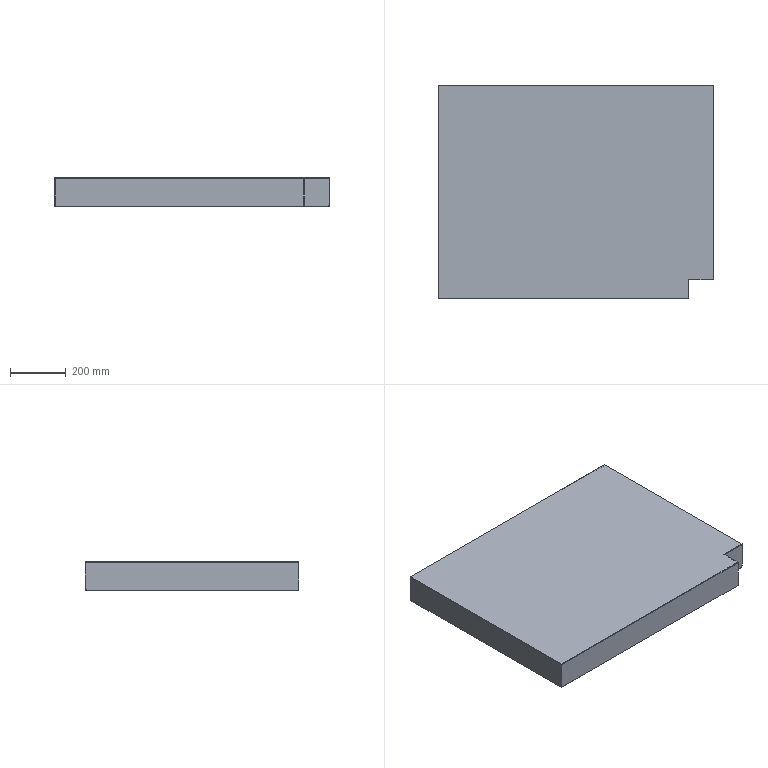Part | STEP file | PN_0054 checkered steel plate 2_Default<As Machined> | 3 solids | 29 faces | box 991 x 771 x 103 mm | volume 2887790 mm3 | plane 26 | cylinder 3 | commonest cylinder face diameters 20 x3